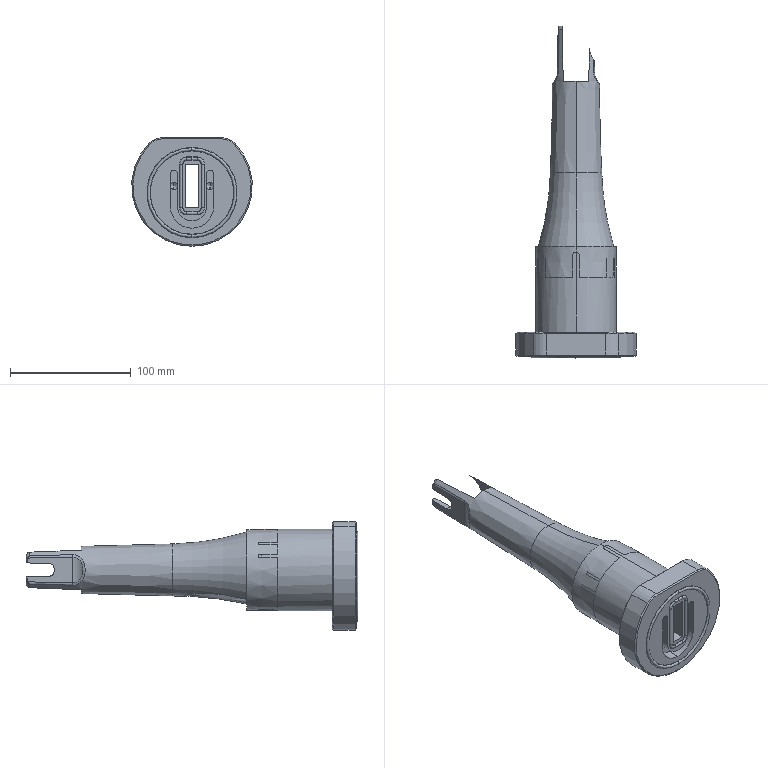Part | STEP file | Core - Tower - Insert 3 - 1 cav | 3 solids | 161 faces | box 100 x 274.891 x 90 mm | volume 522532 mm3 | plane 67 | cylinder 45 | cone 19 | torus 16 | spline 14 | commonest cylinder face diameters 2.5 x10 6 x10 12 x4 2.035 x2 24 x2 24.781 x2